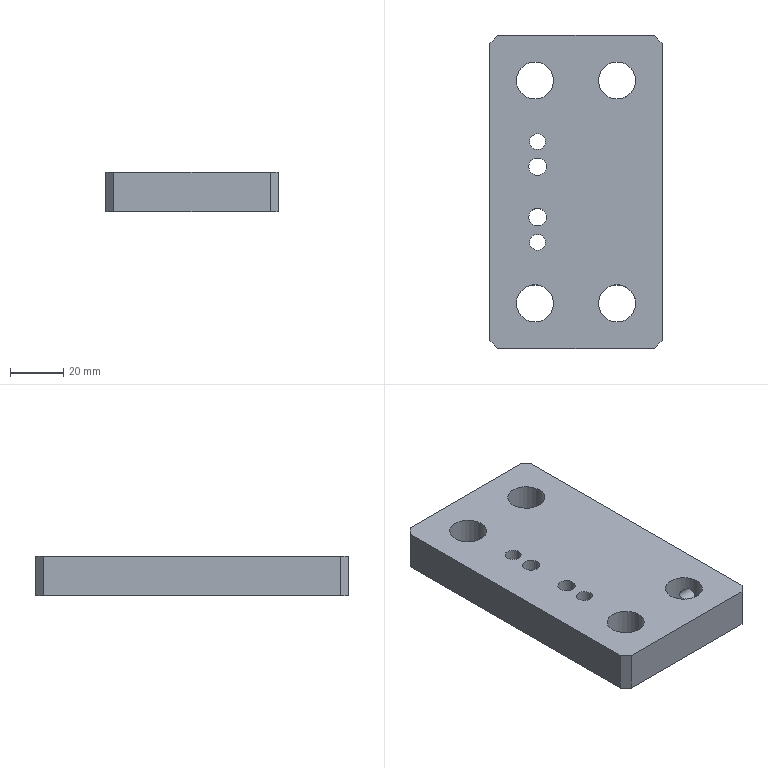Part | NX | features BREP 1 | 1 solid | 26 faces | box 65 x 118 x 15 mm | volume 102149 mm3 | cylinder 13 | plane 12 | cone 1 | commonest cylinder face diameters 14 x4 5 x3 6 x2 6.6 x2 11 x2
STEP:
#1=CARTESIAN_POINT('',(32.5,-38.5,5.));
#2=VERTEX_POINT('',#1);
#3=CARTESIAN_POINT('',(32.5,-38.5,7.5));
#4=DIRECTION('',(1.,0.,0.));
#5=DIRECTION('',(0.,0.,-1.));
#6=AXIS2_PLACEMENT_3D('',#3,#4,#5);
#7=CIRCLE('',#6,2.5);
#8=EDGE_CURVE('',#2,#2,#7,.T.);
#9=ORIENTED_EDGE('',*,*,#8,.F.);
#10=EDGE_LOOP('',(#9));
#11=FACE_BOUND('',#10,.T.);
#12=CARTESIAN_POINT('',(32.5,38.5,5.));
#13=VERTEX_POINT('',#12);
#14=CARTESIAN_POINT('',(32.5,38.5,7.5));
#15=DIRECTION('',(1.,0.,0.));
#16=DIRECTION('',(0.,0.,-1.));
#17=AXIS2_PLACEMENT_3D('',#14,#15,#16);
#18=CIRCLE('',#17,2.5);
#19=EDGE_CURVE('',#13,#13,#18,.T.);
#20=ORIENTED_EDGE('',*,*,#19,.F.);
#21=EDGE_LOOP('',(#20));
#22=FACE_BOUND('',#21,.T.);
#23=CARTESIAN_POINT('',(32.5,-56.,15.));
#24=VERTEX_POINT('',#23);
#25=CARTESIAN_POINT('',(32.5,56.,15.));
#26=VERTEX_POINT('',#25);
#27=CARTESIAN_POINT('',(32.5,59.,15.));
#28=DIRECTION('',(0.,1.,0.));
#29=VECTOR('',#28,1000.);
#30=LINE('',#27,#29);
#31=EDGE_CURVE('',#24,#26,#30,.T.);
#32=ORIENTED_EDGE('',*,*,#31,.F.);
#33=CARTESIAN_POINT('',(32.5,-56.,0.));
#34=VERTEX_POINT('',#33);
#35=CARTESIAN_POINT('',(32.5,-56.,15.));
#36=DIRECTION('',(0.,0.,-1.));
#37=VECTOR('',#36,1000.);
#38=LINE('',#35,#37);
#39=EDGE_CURVE('',#24,#34,#38,.T.);
#40=ORIENTED_EDGE('',*,*,#39,.T.);
#41=CARTESIAN_POINT('',(32.5,56.,0.));
#42=VERTEX_POINT('',#41);
#43=CARTESIAN_POINT('',(32.5,59.,0.));
#44=DIRECTION('',(0.,1.,0.));
#45=VECTOR('',#44,1000.);
#46=LINE('',#43,#45);
#47=EDGE_CURVE('',#34,#42,#46,.T.);
#48=ORIENTED_EDGE('',*,*,#47,.T.);
#49=CARTESIAN_POINT('',(32.5,56.,15.));
#50=DIRECTION('',(0.,0.,1.));
#51=VECTOR('',#50,1000.);
#52=LINE('',#49,#51);
#53=EDGE_CURVE('',#42,#26,#52,.T.);
#54=ORIENTED_EDGE('',*,*,#53,.T.);
#55=EDGE_LOOP('',(#32,#40,#48,#54));
#56=FACE_BOUND('',#55,.T.);
#57=CARTESIAN_POINT('',(32.5,59.,15.));
#58=DIRECTION('',(-1.,0.,0.));
#59=DIRECTION('',(0.,1.,0.));
#60=AXIS2_PLACEMENT_3D('',#57,#58,#59);
#61=PLANE('',#60);
#62=ADVANCED_FACE('',(#11,#22,#56),#61,.F.);
#63=CARTESIAN_POINT('',(0.,59.,10.));
#64=VERTEX_POINT('',#63);
#65=CARTESIAN_POINT('',(0.,59.,7.5));
#66=DIRECTION('',(0.,1.,0.));
#67=DIRECTION('',(0.,0.,1.));
#68=AXIS2_PLACEMENT_3D('',#65,#66,#67);
#69=CIRCLE('',#68,2.5);
#70=EDGE_CURVE('',#64,#64,#69,.T.);
#71=ORIENTED_EDGE('',*,*,#70,.F.);
#72=EDGE_LOOP('',(#71));
#73=FACE_BOUND('',#72,.T.);
#74=CARTESIAN_POINT('',(29.5,59.,0.));
#75=VERTEX_POINT('',#74);
#76=CARTESIAN_POINT('',(-29.5,59.,0.));
#77=VERTEX_POINT('',#76);
#78=CARTESIAN_POINT('',(-32.5,59.,0.));
#79=DIRECTION('',(-1.,0.,0.));
#80=VECTOR('',#79,1000.);
#81=LINE('',#78,#80);
#82=EDGE_CURVE('',#75,#77,#81,.T.);
#83=ORIENTED_EDGE('',*,*,#82,.T.);
#84=CARTESIAN_POINT('',(-29.5,59.,15.));
#85=VERTEX_POINT('',#84);
#86=CARTESIAN_POINT('',(-29.5,59.,15.));
#87=DIRECTION('',(0.,0.,1.));
#88=VECTOR('',#87,1000.);
#89=LINE('',#86,#88);
#90=EDGE_CURVE('',#77,#85,#89,.T.);
#91=ORIENTED_EDGE('',*,*,#90,.T.);
#92=CARTESIAN_POINT('',(29.5,59.,15.));
#93=VERTEX_POINT('',#92);
#94=CARTESIAN_POINT('',(-32.5,59.,15.));
#95=DIRECTION('',(-1.,0.,0.));
#96=VECTOR('',#95,1000.);
#97=LINE('',#94,#96);
#98=EDGE_CURVE('',#93,#85,#97,.T.);
#99=ORIENTED_EDGE('',*,*,#98,.F.);
#100=CARTESIAN_POINT('',(29.5,59.,15.));
#101=DIRECTION('',(0.,0.,-1.));
#102=VECTOR('',#101,1000.);
#103=LINE('',#100,#102);
#104=EDGE_CURVE('',#93,#75,#103,.T.);
#105=ORIENTED_EDGE('',*,*,#104,.T.);
#106=EDGE_LOOP('',(#83,#91,#99,#105));
#107=FACE_BOUND('',#106,.T.);
#108=CARTESIAN_POINT('',(-32.5,59.,15.));
#109=DIRECTION('',(0.,-1.,0.));
#110=DIRECTION('',(0.,0.,1.));
#111=AXIS2_PLACEMENT_3D('',#108,#109,#110);
#112=PLANE('',#111);
#113=ADVANCED_FACE('',(#73,#107),#112,.F.);
#114=CARTESIAN_POINT('',(-32.5,56.,0.));
#115=VERTEX_POINT('',#114);
#116=CARTESIAN_POINT('',(-32.5,-56.,0.));
#117=VERTEX_POINT('',#116);
#118=CARTESIAN_POINT('',(-32.5,59.,0.));
#119=DIRECTION('',(0.,-1.,0.));
#120=VECTOR('',#119,1000.);
#121=LINE('',#118,#120);
#122=EDGE_CURVE('',#115,#117,#121,.T.);
#123=ORIENTED_EDGE('',*,*,#122,.T.);
#124=CARTESIAN_POINT('',(-32.5,-56.,15.));
#125=VERTEX_POINT('',#124);
#126=CARTESIAN_POINT('',(-32.5,-56.,15.));
#127=DIRECTION('',(0.,0.,1.));
#128=VECTOR('',#127,1000.);
#129=LINE('',#126,#128);
#130=EDGE_CURVE('',#117,#125,#129,.T.);
#131=ORIENTED_EDGE('',*,*,#130,.T.);
#132=CARTESIAN_POINT('',(-32.5,56.,15.));
#133=VERTEX_POINT('',#132);
#134=CARTESIAN_POINT('',(-32.5,59.,15.));
#135=DIRECTION('',(0.,-1.,0.));
#136=VECTOR('',#135,1000.);
#137=LINE('',#134,#136);
#138=EDGE_CURVE('',#133,#125,#137,.T.);
#139=ORIENTED_EDGE('',*,*,#138,.F.);
#140=CARTESIAN_POINT('',(-32.5,56.,15.));
#141=DIRECTION('',(0.,0.,-1.));
#142=VECTOR('',#141,1000.);
#143=LINE('',#140,#142);
#144=EDGE_CURVE('',#133,#115,#143,.T.);
#145=ORIENTED_EDGE('',*,*,#144,.T.);
#146=EDGE_LOOP('',(#123,#131,#139,#145));
#147=FACE_BOUND('',#146,.T.);
#148=CARTESIAN_POINT('',(-32.5,59.,15.));
#149=DIRECTION('',(1.,0.,0.));
#150=DIRECTION('',(0.,-1.,0.));
#151=AXIS2_PLACEMENT_3D('',#148,#149,#150);
#152=PLANE('',#151);
#153=ADVANCED_FACE('',(#147),#152,.F.);
#154=CARTESIAN_POINT('',(-29.5,-59.,15.));
#155=VERTEX_POINT('',#154);
#156=CARTESIAN_POINT('',(29.5,-59.,15.));
#157=VERTEX_POINT('',#156);
#158=CARTESIAN_POINT('',(-32.5,-59.,15.));
#159=DIRECTION('',(1.,0.,0.));
#160=VECTOR('',#159,1000.);
#161=LINE('',#158,#160);
#162=EDGE_CURVE('',#155,#157,#161,.T.);
#163=ORIENTED_EDGE('',*,*,#162,.F.);
#164=CARTESIAN_POINT('',(-29.5,-59.,0.));
#165=VERTEX_POINT('',#164);
#166=CARTESIAN_POINT('',(-29.5,-59.,15.));
#167=DIRECTION('',(0.,0.,-1.));
#168=VECTOR('',#167,1000.);
#169=LINE('',#166,#168);
#170=EDGE_CURVE('',#155,#165,#169,.T.);
#171=ORIENTED_EDGE('',*,*,#170,.T.);
#172=CARTESIAN_POINT('',(29.5,-59.,0.));
#173=VERTEX_POINT('',#172);
#174=CARTESIAN_POINT('',(-32.5,-59.,0.));
#175=DIRECTION('',(1.,0.,0.));
#176=VECTOR('',#175,1000.);
#177=LINE('',#174,#176);
#178=EDGE_CURVE('',#165,#173,#177,.T.);
#179=ORIENTED_EDGE('',*,*,#178,.T.);
#180=CARTESIAN_POINT('',(29.5,-59.,15.));
#181=DIRECTION('',(0.,0.,1.));
#182=VECTOR('',#181,1000.);
#183=LINE('',#180,#182);
#184=EDGE_CURVE('',#173,#157,#183,.T.);
#185=ORIENTED_EDGE('',*,*,#184,.T.);
#186=EDGE_LOOP('',(#163,#171,#179,#185));
#187=FACE_BOUND('',#186,.T.);
#188=CARTESIAN_POINT('',(-32.5,-59.,15.));
#189=DIRECTION('',(0.,1.,0.));
#190=DIRECTION('',(0.,0.,-1.));
#191=AXIS2_PLACEMENT_3D('',#188,#189,#190);
#192=PLANE('',#191);
#193=ADVANCED_FACE('',(#187),#192,.F.);
#194=CARTESIAN_POINT('',(-17.8,9.5,15.));
#195=VERTEX_POINT('',#194);
#196=CARTESIAN_POINT('',(-14.5,9.5,15.));
#197=DIRECTION('',(0.,0.,-1.));
#198=DIRECTION('',(-1.,0.,0.));
#199=AXIS2_PLACEMENT_3D('',#196,#197,#198);
#200=CIRCLE('',#199,3.3);
#201=EDGE_CURVE('',#195,#195,#200,.T.);
#202=ORIENTED_EDGE('',*,*,#201,.T.);
#203=EDGE_LOOP('',(#202));
#204=FACE_BOUND('',#203,.T.);
#205=CARTESIAN_POINT('',(-17.8,-9.5,15.));
#206=VERTEX_POINT('',#205);
#207=CARTESIAN_POINT('',(-14.5,-9.5,15.));
#208=DIRECTION('',(0.,0.,-1.));
#209=DIRECTION('',(-1.,0.,0.));
#210=AXIS2_PLACEMENT_3D('',#207,#208,#209);
#211=CIRCLE('',#210,3.3);
#212=EDGE_CURVE('',#206,#206,#211,.T.);
#213=ORIENTED_EDGE('',*,*,#212,.T.);
#214=EDGE_LOOP('',(#213));
#215=FACE_BOUND('',#214,.T.);
#216=CARTESIAN_POINT('',(-11.5,19.,15.));
#217=VERTEX_POINT('',#216);
#218=CARTESIAN_POINT('',(-14.5,19.,15.));
#219=DIRECTION('',(0.,0.,1.));
#220=DIRECTION('',(1.,0.,0.));
#221=AXIS2_PLACEMENT_3D('',#218,#219,#220);
#222=CIRCLE('',#221,3.);
#223=EDGE_CURVE('',#217,#217,#222,.T.);
#224=ORIENTED_EDGE('',*,*,#223,.F.);
#225=EDGE_LOOP('',(#224));
#226=FACE_BOUND('',#225,.T.);
#227=CARTESIAN_POINT('',(-11.5,-19.,15.));
#228=VERTEX_POINT('',#227);
#229=CARTESIAN_POINT('',(-14.5,-19.,15.));
#230=DIRECTION('',(0.,0.,1.));
#231=DIRECTION('',(1.,0.,0.));
#232=AXIS2_PLACEMENT_3D('',#229,#230,#231);
#233=CIRCLE('',#232,3.);
#234=EDGE_CURVE('',#228,#228,#233,.T.);
#235=ORIENTED_EDGE('',*,*,#234,.F.);
#236=EDGE_LOOP('',(#235));
#237=FACE_BOUND('',#236,.T.);
#238=CARTESIAN_POINT('',(-8.5,42.,15.));
#239=VERTEX_POINT('',#238);
#240=CARTESIAN_POINT('',(-15.5,42.,15.));
#241=DIRECTION('',(0.,0.,1.));
#242=DIRECTION('',(1.,0.,0.));
#243=AXIS2_PLACEMENT_3D('',#240,#241,#242);
#244=CIRCLE('',#243,7.);
#245=EDGE_CURVE('',#239,#239,#244,.T.);
#246=ORIENTED_EDGE('',*,*,#245,.F.);
#247=EDGE_LOOP('',(#246));
#248=FACE_BOUND('',#247,.T.);
#249=CARTESIAN_POINT('',(22.5,42.,15.));
#250=VERTEX_POINT('',#249);
#251=CARTESIAN_POINT('',(15.5,42.,15.));
#252=DIRECTION('',(0.,0.,1.));
#253=DIRECTION('',(1.,0.,0.));
#254=AXIS2_PLACEMENT_3D('',#251,#252,#253);
#255=CIRCLE('',#254,7.);
#256=EDGE_CURVE('',#250,#250,#255,.T.);
#257=ORIENTED_EDGE('',*,*,#256,.F.);
#258=EDGE_LOOP('',(#257));
#259=FACE_BOUND('',#258,.T.);
#260=CARTESIAN_POINT('',(-8.5,-42.,15.));
#261=VERTEX_POINT('',#260);
#262=CARTESIAN_POINT('',(-15.5,-42.,15.));
#263=DIRECTION('',(0.,0.,1.));
#264=DIRECTION('',(1.,0.,0.));
#265=AXIS2_PLACEMENT_3D('',#262,#263,#264);
#266=CIRCLE('',#265,7.);
#267=EDGE_CURVE('',#261,#261,#266,.T.);
#268=ORIENTED_EDGE('',*,*,#267,.F.);
#269=EDGE_LOOP('',(#268));
#270=FACE_BOUND('',#269,.T.);
#271=CARTESIAN_POINT('',(22.5,-42.,15.));
#272=VERTEX_POINT('',#271);
#273=CARTESIAN_POINT('',(15.5,-42.,15.));
#274=DIRECTION('',(0.,0.,1.));
#275=DIRECTION('',(1.,0.,0.));
#276=AXIS2_PLACEMENT_3D('',#273,#274,#275);
#277=CIRCLE('',#276,7.);
#278=EDGE_CURVE('',#272,#272,#277,.T.);
#279=ORIENTED_EDGE('',*,*,#278,.F.);
#280=EDGE_LOOP('',(#279));
#281=FACE_BOUND('',#280,.T.);
#282=ORIENTED_EDGE('',*,*,#138,.T.);
#283=CARTESIAN_POINT('',(-44.25,-44.25,15.));
#284=DIRECTION('',(0.7071,-0.7071,0.));
#285=VECTOR('',#284,1000.);
#286=LINE('',#283,#285);
#287=EDGE_CURVE('',#125,#155,#286,.T.);
#288=ORIENTED_EDGE('',*,*,#287,.T.);
#289=ORIENTED_EDGE('',*,*,#162,.T.);
#290=CARTESIAN_POINT('',(44.25,-44.25,15.));
#291=DIRECTION('',(0.7071,0.7071,0.));
#292=VECTOR('',#291,1000.);
#293=LINE('',#290,#292);
#294=EDGE_CURVE('',#157,#24,#293,.T.);
#295=ORIENTED_EDGE('',*,*,#294,.T.);
#296=ORIENTED_EDGE('',*,*,#31,.T.);
#297=CARTESIAN_POINT('',(44.25,44.25,15.));
#298=DIRECTION('',(-0.7071,0.7071,0.));
#299=VECTOR('',#298,1000.);
#300=LINE('',#297,#299);
#301=EDGE_CURVE('',#26,#93,#300,.T.);
#302=ORIENTED_EDGE('',*,*,#301,.T.);
#303=ORIENTED_EDGE('',*,*,#98,.T.);
#304=CARTESIAN_POINT('',(-44.25,44.25,15.));
#305=DIRECTION('',(-0.7071,-0.7071,0.));
#306=VECTOR('',#305,1000.);
#307=LINE('',#304,#306);
#308=EDGE_CURVE('',#85,#133,#307,.T.);
#309=ORIENTED_EDGE('',*,*,#308,.T.);
#310=EDGE_LOOP('',(#282,#288,#289,#295,#296,#302,#303,#309));
#311=FACE_BOUND('',#310,.T.);
#312=CARTESIAN_POINT('',(0.,0.,15.));
#313=DIRECTION('',(0.,0.,1.));
#314=DIRECTION('',(-1.,0.,0.));
#315=AXIS2_PLACEMENT_3D('',#312,#313,#314);
#316=PLANE('',#315);
#317=ADVANCED_FACE('',(#204,#215,#226,#237,#248,#259,#270,#281,#311),#316,.T.);
#318=CARTESIAN_POINT('',(-20.,9.5,0.));
#319=VERTEX_POINT('',#318);
#320=CARTESIAN_POINT('',(-14.5,9.5,0.));
#321=DIRECTION('',(0.,0.,-1.));
#322=DIRECTION('',(-1.,0.,0.));
#323=AXIS2_PLACEMENT_3D('',#320,#321,#322);
#324=CIRCLE('',#323,5.5);
#325=EDGE_CURVE('',#319,#319,#324,.T.);
#326=ORIENTED_EDGE('',*,*,#325,.F.);
#327=EDGE_LOOP('',(#326));
#328=FACE_BOUND('',#327,.T.);
#329=CARTESIAN_POINT('',(-20.,-9.5,0.));
#330=VERTEX_POINT('',#329);
#331=CARTESIAN_POINT('',(-14.5,-9.5,0.));
#332=DIRECTION('',(0.,0.,-1.));
#333=DIRECTION('',(-1.,0.,0.));
#334=AXIS2_PLACEMENT_3D('',#331,#332,#333);
#335=CIRCLE('',#334,5.5);
#336=EDGE_CURVE('',#330,#330,#335,.T.);
#337=ORIENTED_EDGE('',*,*,#336,.F.);
#338=EDGE_LOOP('',(#337));
#339=FACE_BOUND('',#338,.T.);
#340=CARTESIAN_POINT('',(-11.5,19.,0.));
#341=VERTEX_POINT('',#340);
#342=CARTESIAN_POINT('',(-14.5,19.,0.));
#343=DIRECTION('',(0.,0.,1.));
#344=DIRECTION('',(1.,0.,0.));
#345=AXIS2_PLACEMENT_3D('',#342,#343,#344);
#346=CIRCLE('',#345,3.);
#347=EDGE_CURVE('',#341,#341,#346,.T.);
#348=ORIENTED_EDGE('',*,*,#347,.T.);
#349=EDGE_LOOP('',(#348));
#350=FACE_BOUND('',#349,.T.);
#351=CARTESIAN_POINT('',(-11.5,-19.,0.));
#352=VERTEX_POINT('',#351);
#353=CARTESIAN_POINT('',(-14.5,-19.,0.));
#354=DIRECTION('',(0.,0.,1.));
#355=DIRECTION('',(1.,0.,0.));
#356=AXIS2_PLACEMENT_3D('',#353,#354,#355);
#357=CIRCLE('',#356,3.);
#358=EDGE_CURVE('',#352,#352,#357,.T.);
#359=ORIENTED_EDGE('',*,*,#358,.T.);
#360=EDGE_LOOP('',(#359));
#361=FACE_BOUND('',#360,.T.);
#362=CARTESIAN_POINT('',(-8.5,42.,0.));
#363=VERTEX_POINT('',#362);
#364=CARTESIAN_POINT('',(-15.5,42.,0.));
#365=DIRECTION('',(0.,0.,1.));
#366=DIRECTION('',(1.,0.,0.));
#367=AXIS2_PLACEMENT_3D('',#364,#365,#366);
#368=CIRCLE('',#367,7.);
#369=EDGE_CURVE('',#363,#363,#368,.T.);
#370=ORIENTED_EDGE('',*,*,#369,.T.);
#371=EDGE_LOOP('',(#370));
#372=FACE_BOUND('',#371,.T.);
#373=CARTESIAN_POINT('',(22.5,42.,0.));
#374=VERTEX_POINT('',#373);
#375=CARTESIAN_POINT('',(15.5,42.,0.));
#376=DIRECTION('',(0.,0.,1.));
#377=DIRECTION('',(1.,0.,0.));
#378=AXIS2_PLACEMENT_3D('',#375,#376,#377);
#379=CIRCLE('',#378,7.);
#380=EDGE_CURVE('',#374,#374,#379,.T.);
#381=ORIENTED_EDGE('',*,*,#380,.T.);
#382=EDGE_LOOP('',(#381));
#383=FACE_BOUND('',#382,.T.);
#384=CARTESIAN_POINT('',(-8.5,-42.,0.));
#385=VERTEX_POINT('',#384);
#386=CARTESIAN_POINT('',(-15.5,-42.,0.));
#387=DIRECTION('',(0.,0.,1.));
#388=DIRECTION('',(1.,0.,0.));
#389=AXIS2_PLACEMENT_3D('',#386,#387,#388);
#390=CIRCLE('',#389,7.);
#391=EDGE_CURVE('',#385,#385,#390,.T.);
#392=ORIENTED_EDGE('',*,*,#391,.T.);
#393=EDGE_LOOP('',(#392));
#394=FACE_BOUND('',#393,.T.);
#395=CARTESIAN_POINT('',(22.5,-42.,0.));
#396=VERTEX_POINT('',#395);
#397=CARTESIAN_POINT('',(15.5,-42.,0.));
#398=DIRECTION('',(0.,0.,1.));
#399=DIRECTION('',(1.,0.,0.));
#400=AXIS2_PLACEMENT_3D('',#397,#398,#399);
#401=CIRCLE('',#400,7.);
#402=EDGE_CURVE('',#396,#396,#401,.T.);
#403=ORIENTED_EDGE('',*,*,#402,.T.);
#404=EDGE_LOOP('',(#403));
#405=FACE_BOUND('',#404,.T.);
#406=ORIENTED_EDGE('',*,*,#178,.F.);
#407=CARTESIAN_POINT('',(-29.5,-59.,0.));
#408=DIRECTION('',(-0.7071,0.7071,0.));
#409=VECTOR('',#408,1000.);
#410=LINE('',#407,#409);
#411=EDGE_CURVE('',#165,#117,#410,.T.);
#412=ORIENTED_EDGE('',*,*,#411,.T.);
#413=ORIENTED_EDGE('',*,*,#122,.F.);
#414=CARTESIAN_POINT('',(-32.5,56.,0.));
#415=DIRECTION('',(0.7071,0.7071,0.));
#416=VECTOR('',#415,1000.);
#417=LINE('',#414,#416);
#418=EDGE_CURVE('',#115,#77,#417,.T.);
#419=ORIENTED_EDGE('',*,*,#418,.T.);
#420=ORIENTED_EDGE('',*,*,#82,.F.);
#421=CARTESIAN_POINT('',(29.5,59.,0.));
#422=DIRECTION('',(0.7071,-0.7071,0.));
#423=VECTOR('',#422,1000.);
#424=LINE('',#421,#423);
#425=EDGE_CURVE('',#75,#42,#424,.T.);
#426=ORIENTED_EDGE('',*,*,#425,.T.);
#427=ORIENTED_EDGE('',*,*,#47,.F.);
#428=CARTESIAN_POINT('',(32.5,-56.,0.));
#429=DIRECTION('',(-0.7071,-0.7071,0.));
#430=VECTOR('',#429,1000.);
#431=LINE('',#428,#430);
#432=EDGE_CURVE('',#34,#173,#431,.T.);
#433=ORIENTED_EDGE('',*,*,#432,.T.);
#434=EDGE_LOOP('',(#406,#412,#413,#419,#420,#426,#427,#433));
#435=FACE_BOUND('',#434,.T.);
#436=CARTESIAN_POINT('',(0.,0.,0.));
#437=DIRECTION('',(0.,0.,1.));
#438=DIRECTION('',(-1.,0.,0.));
#439=AXIS2_PLACEMENT_3D('',#436,#437,#438);
#440=PLANE('',#439);
#441=ADVANCED_FACE('',(#328,#339,#350,#361,#372,#383,#394,#405,#435),#440,.F.);
#442=CARTESIAN_POINT('',(21.562,-38.5,5.));
#443=VERTEX_POINT('',#442);
#444=CARTESIAN_POINT('',(22.415,-40.562,5.55));
#445=CARTESIAN_POINT('',(21.797,-38.777,4.873));
#446=CARTESIAN_POINT('',(20.968,-37.589,5.119));
#447=CARTESIAN_POINT('',(20.271,-36.848,5.562));
#448=CARTESIAN_POINT('',(19.587,-36.297,6.21));
#449=CARTESIAN_POINT('',(19.006,-35.94,7.157));
#450=CARTESIAN_POINT('',(19.213,-36.059,8.31));
#451=CARTESIAN_POINT('',(19.88,-36.514,9.092));
#452=CARTESIAN_POINT('',(20.572,-37.144,9.655));
#453=CARTESIAN_POINT('',(21.469,-38.21,10.11));
#454=CARTESIAN_POINT('',(22.306,-39.988,9.896));
#455=CARTESIAN_POINT('',(22.458,-41.332,7.866));
#456=CARTESIAN_POINT('',(22.415,-40.562,5.55));
#457=CARTESIAN_POINT('',(21.797,-38.777,4.873));
#458=CARTESIAN_POINT('',(20.968,-37.589,5.119));
#459=B_SPLINE_CURVE_WITH_KNOTS('',3,(#444,#445,#446,#447,#448,#449,#450,#451,#452,#453,#454,#455,#456,#457,#458),.UNSPECIFIED.,.T.,.F.,(1,1,1,1,1,1,1,1,1,1,1,1,1,1,1,1,1,1,1),(-0.006513,-0.004342,-0.002171,0.,0.001085,0.002171,0.003256,0.004342,0.005427,0.006513,0.007598,0.008683,0.01085,0.01303,0.0152,0.01737,0.01845,0.01954,0.02062),.UNSPECIFIED.);
#460=EDGE_CURVE('',#443,#443,#459,.T.);
#461=ORIENTED_EDGE('',*,*,#460,.T.);
#462=EDGE_LOOP('',(#461));
#463=FACE_BOUND('',#462,.T.);
#464=ORIENTED_EDGE('',*,*,#402,.F.);
#465=EDGE_LOOP('',(#464));
#466=FACE_BOUND('',#465,.T.);
#467=ORIENTED_EDGE('',*,*,#278,.T.);
#468=EDGE_LOOP('',(#467));
#469=FACE_BOUND('',#468,.T.);
#470=CARTESIAN_POINT('',(15.5,-42.,15.));
#471=DIRECTION('',(0.,0.,1.));
#472=DIRECTION('',(-1.,0.,0.));
#473=AXIS2_PLACEMENT_3D('',#470,#471,#472);
#474=CYLINDRICAL_SURFACE('',#473,7.);
#475=ADVANCED_FACE('',(#463,#466,#469),#474,.F.);
#476=ORIENTED_EDGE('',*,*,#391,.F.);
#477=EDGE_LOOP('',(#476));
#478=FACE_BOUND('',#477,.T.);
#479=ORIENTED_EDGE('',*,*,#267,.T.);
#480=EDGE_LOOP('',(#479));
#481=FACE_BOUND('',#480,.T.);
#482=CARTESIAN_POINT('',(-15.5,-42.,15.));
#483=DIRECTION('',(0.,0.,1.));
#484=DIRECTION('',(-1.,0.,0.));
#485=AXIS2_PLACEMENT_3D('',#482,#483,#484);
#486=CYLINDRICAL_SURFACE('',#485,7.);
#487=ADVANCED_FACE('',(#478,#481),#486,.F.);
#488=CARTESIAN_POINT('',(21.562,38.5,5.));
#489=VERTEX_POINT('',#488);
#490=CARTESIAN_POINT('',(20.964,37.584,5.121));
#491=CARTESIAN_POINT('',(21.8,38.781,4.873));
#492=CARTESIAN_POINT('',(22.412,40.552,5.543));
#493=CARTESIAN_POINT('',(22.458,41.332,7.855));
#494=CARTESIAN_POINT('',(22.31,40.004,9.885));
#495=CARTESIAN_POINT('',(21.475,38.218,10.112));
#496=CARTESIAN_POINT('',(20.573,37.144,9.656));
#497=CARTESIAN_POINT('',(19.877,36.511,9.089));
#498=CARTESIAN_POINT('',(19.211,36.057,8.307));
#499=CARTESIAN_POINT('',(19.007,35.941,7.152));
#500=CARTESIAN_POINT('',(19.588,36.298,6.209));
#501=CARTESIAN_POINT('',(20.272,36.849,5.562));
#502=CARTESIAN_POINT('',(20.964,37.584,5.121));
#503=CARTESIAN_POINT('',(21.8,38.781,4.873));
#504=CARTESIAN_POINT('',(22.412,40.552,5.543));
#505=B_SPLINE_CURVE_WITH_KNOTS('',3,(#490,#491,#492,#493,#494,#495,#496,#497,#498,#499,#500,#501,#502,#503,#504),.UNSPECIFIED.,.T.,.F.,(1,1,1,1,1,1,1,1,1,1,1,1,1,1,1,1,1,1,1),(-0.003271,-0.002181,-0.00109,0.,0.002181,0.004362,0.006543,0.008723,0.009814,0.0109,0.01199,0.01309,0.01418,0.01527,0.01636,0.01745,0.01963,0.02181,0.02399),.UNSPECIFIED.);
#506=EDGE_CURVE('',#489,#489,#505,.T.);
#507=ORIENTED_EDGE('',*,*,#506,.T.);
#508=EDGE_LOOP('',(#507));
#509=FACE_BOUND('',#508,.T.);
#510=ORIENTED_EDGE('',*,*,#380,.F.);
#511=EDGE_LOOP('',(#510));
#512=FACE_BOUND('',#511,.T.);
#513=ORIENTED_EDGE('',*,*,#256,.T.);
#514=EDGE_LOOP('',(#513));
#515=FACE_BOUND('',#514,.T.);
#516=CARTESIAN_POINT('',(15.5,42.,15.));
#517=DIRECTION('',(0.,0.,1.));
#518=DIRECTION('',(-1.,0.,0.));
#519=AXIS2_PLACEMENT_3D('',#516,#517,#518);
#520=CYLINDRICAL_SURFACE('',#519,7.);
#521=ADVANCED_FACE('',(#509,#512,#515),#520,.F.);
#522=ORIENTED_EDGE('',*,*,#369,.F.);
#523=EDGE_LOOP('',(#522));
#524=FACE_BOUND('',#523,.T.);
#525=ORIENTED_EDGE('',*,*,#245,.T.);
#526=EDGE_LOOP('',(#525));
#527=FACE_BOUND('',#526,.T.);
#528=CARTESIAN_POINT('',(-15.5,42.,15.));
#529=DIRECTION('',(0.,0.,1.));
#530=DIRECTION('',(-1.,0.,0.));
#531=AXIS2_PLACEMENT_3D('',#528,#529,#530);
#532=CYLINDRICAL_SURFACE('',#531,7.);
#533=ADVANCED_FACE('',(#524,#527),#532,.F.);
#534=ORIENTED_EDGE('',*,*,#287,.F.);
#535=ORIENTED_EDGE('',*,*,#130,.F.);
#536=ORIENTED_EDGE('',*,*,#411,.F.);
#537=ORIENTED_EDGE('',*,*,#170,.F.);
#538=EDGE_LOOP('',(#534,#535,#536,#537));
#539=FACE_BOUND('',#538,.T.);
#540=CARTESIAN_POINT('',(-29.5,-59.,15.));
#541=DIRECTION('',(0.7071,0.7071,0.));
#542=DIRECTION('',(0.,0.,1.));
#543=AXIS2_PLACEMENT_3D('',#540,#541,#542);
#544=PLANE('',#543);
#545=ADVANCED_FACE('',(#539),#544,.F.);
#546=ORIENTED_EDGE('',*,*,#294,.F.);
#547=ORIENTED_EDGE('',*,*,#184,.F.);
#548=ORIENTED_EDGE('',*,*,#432,.F.);
#549=ORIENTED_EDGE('',*,*,#39,.F.);
#550=EDGE_LOOP('',(#546,#547,#548,#549));
#551=FACE_BOUND('',#550,.T.);
#552=CARTESIAN_POINT('',(32.5,-56.,15.));
#553=DIRECTION('',(-0.7071,0.7071,0.));
#554=DIRECTION('',(0.,0.,1.));
#555=AXIS2_PLACEMENT_3D('',#552,#553,#554);
#556=PLANE('',#555);
#557=ADVANCED_FACE('',(#551),#556,.F.);
#558=ORIENTED_EDGE('',*,*,#308,.F.);
#559=ORIENTED_EDGE('',*,*,#90,.F.);
#560=ORIENTED_EDGE('',*,*,#418,.F.);
#561=ORIENTED_EDGE('',*,*,#144,.F.);
#562=EDGE_LOOP('',(#558,#559,#560,#561));
#563=FACE_BOUND('',#562,.T.);
#564=CARTESIAN_POINT('',(-32.5,56.,15.));
#565=DIRECTION('',(0.7071,-0.7071,0.));
#566=DIRECTION('',(0.,0.,1.));
#567=AXIS2_PLACEMENT_3D('',#564,#565,#566);
#568=PLANE('',#567);
#569=ADVANCED_FACE('',(#563),#568,.F.);
#570=ORIENTED_EDGE('',*,*,#301,.F.);
#571=ORIENTED_EDGE('',*,*,#53,.F.);
#572=ORIENTED_EDGE('',*,*,#425,.F.);
#573=ORIENTED_EDGE('',*,*,#104,.F.);
#574=EDGE_LOOP('',(#570,#571,#572,#573));
#575=FACE_BOUND('',#574,.T.);
#576=CARTESIAN_POINT('',(29.5,59.,15.));
#577=DIRECTION('',(-0.7071,-0.7071,0.));
#578=DIRECTION('',(0.,0.,1.));
#579=AXIS2_PLACEMENT_3D('',#576,#577,#578);
#580=PLANE('',#579);
#581=ADVANCED_FACE('',(#575),#580,.F.);
#582=ORIENTED_EDGE('',*,*,#358,.F.);
#583=EDGE_LOOP('',(#582));
#584=FACE_BOUND('',#583,.T.);
#585=ORIENTED_EDGE('',*,*,#234,.T.);
#586=EDGE_LOOP('',(#585));
#587=FACE_BOUND('',#586,.T.);
#588=CARTESIAN_POINT('',(-14.5,-19.,15.));
#589=DIRECTION('',(0.,0.,1.));
#590=DIRECTION('',(-1.,0.,0.));
#591=AXIS2_PLACEMENT_3D('',#588,#589,#590);
#592=CYLINDRICAL_SURFACE('',#591,3.);
#593=ADVANCED_FACE('',(#584,#587),#592,.F.);
#594=ORIENTED_EDGE('',*,*,#347,.F.);
#595=EDGE_LOOP('',(#594));
#596=FACE_BOUND('',#595,.T.);
#597=ORIENTED_EDGE('',*,*,#223,.T.);
#598=EDGE_LOOP('',(#597));
#599=FACE_BOUND('',#598,.T.);
#600=CARTESIAN_POINT('',(-14.5,19.,15.));
#601=DIRECTION('',(0.,0.,1.));
#602=DIRECTION('',(-1.,0.,0.));
#603=AXIS2_PLACEMENT_3D('',#600,#601,#602);
#604=CYLINDRICAL_SURFACE('',#603,3.);
#605=ADVANCED_FACE('',(#596,#599),#604,.F.);
#606=ORIENTED_EDGE('',*,*,#212,.F.);
#607=EDGE_LOOP('',(#606));
#608=FACE_BOUND('',#607,.T.);
#609=CARTESIAN_POINT('',(-17.8,-9.5,6.4));
#610=VERTEX_POINT('',#609);
#611=CARTESIAN_POINT('',(-14.5,-9.5,6.4));
#612=DIRECTION('',(0.,0.,-1.));
#613=DIRECTION('',(-1.,0.,0.));
#614=AXIS2_PLACEMENT_3D('',#611,#612,#613);
#615=CIRCLE('',#614,3.3);
#616=EDGE_CURVE('',#610,#610,#615,.T.);
#617=ORIENTED_EDGE('',*,*,#616,.T.);
#618=EDGE_LOOP('',(#617));
#619=FACE_BOUND('',#618,.T.);
#620=CARTESIAN_POINT('',(-14.5,-9.5,0.));
#621=DIRECTION('',(0.,0.,-1.));
#622=DIRECTION('',(1.,0.,0.));
#623=AXIS2_PLACEMENT_3D('',#620,#621,#622);
#624=CYLINDRICAL_SURFACE('',#623,3.3);
#625=ADVANCED_FACE('',(#608,#619),#624,.F.);
#626=ORIENTED_EDGE('',*,*,#616,.F.);
#627=EDGE_LOOP('',(#626));
#628=FACE_BOUND('',#627,.T.);
#629=CARTESIAN_POINT('',(-20.,-9.5,6.4));
#630=VERTEX_POINT('',#629);
#631=CARTESIAN_POINT('',(-14.5,-9.5,6.4));
#632=DIRECTION('',(0.,0.,-1.));
#633=DIRECTION('',(-1.,0.,0.));
#634=AXIS2_PLACEMENT_3D('',#631,#632,#633);
#635=CIRCLE('',#634,5.5);
#636=EDGE_CURVE('',#630,#630,#635,.T.);
#637=ORIENTED_EDGE('',*,*,#636,.T.);
#638=EDGE_LOOP('',(#637));
#639=FACE_BOUND('',#638,.T.);
#640=CARTESIAN_POINT('',(-11.2,-9.5,6.4));
#641=DIRECTION('',(0.,0.,1.));
#642=DIRECTION('',(-1.,0.,0.));
#643=AXIS2_PLACEMENT_3D('',#640,#641,#642);
#644=PLANE('',#643);
#645=ADVANCED_FACE('',(#628,#639),#644,.F.);
#646=ORIENTED_EDGE('',*,*,#636,.F.);
#647=EDGE_LOOP('',(#646));
#648=FACE_BOUND('',#647,.T.);
#649=ORIENTED_EDGE('',*,*,#336,.T.);
#650=EDGE_LOOP('',(#649));
#651=FACE_BOUND('',#650,.T.);
#652=CARTESIAN_POINT('',(-14.5,-9.5,0.));
#653=DIRECTION('',(0.,0.,-1.));
#654=DIRECTION('',(1.,0.,0.));
#655=AXIS2_PLACEMENT_3D('',#652,#653,#654);
#656=CYLINDRICAL_SURFACE('',#655,5.5);
#657=ADVANCED_FACE('',(#648,#651),#656,.F.);
#658=ORIENTED_EDGE('',*,*,#201,.F.);
#659=EDGE_LOOP('',(#658));
#660=FACE_BOUND('',#659,.T.);
#661=CARTESIAN_POINT('',(-17.8,9.5,6.4));
#662=VERTEX_POINT('',#661);
#663=CARTESIAN_POINT('',(-14.5,9.5,6.4));
#664=DIRECTION('',(0.,0.,-1.));
#665=DIRECTION('',(-1.,0.,0.));
#666=AXIS2_PLACEMENT_3D('',#663,#664,#665);
#667=CIRCLE('',#666,3.3);
#668=EDGE_CURVE('',#662,#662,#667,.T.);
#669=ORIENTED_EDGE('',*,*,#668,.T.);
#670=EDGE_LOOP('',(#669));
#671=FACE_BOUND('',#670,.T.);
#672=CARTESIAN_POINT('',(-14.5,9.5,0.));
#673=DIRECTION('',(0.,0.,-1.));
#674=DIRECTION('',(1.,0.,0.));
#675=AXIS2_PLACEMENT_3D('',#672,#673,#674);
#676=CYLINDRICAL_SURFACE('',#675,3.3);
#677=ADVANCED_FACE('',(#660,#671),#676,.F.);
#678=ORIENTED_EDGE('',*,*,#668,.F.);
#679=EDGE_LOOP('',(#678));
#680=FACE_BOUND('',#679,.T.);
#681=CARTESIAN_POINT('',(-20.,9.5,6.4));
#682=VERTEX_POINT('',#681);
#683=CARTESIAN_POINT('',(-14.5,9.5,6.4));
#684=DIRECTION('',(0.,0.,-1.));
#685=DIRECTION('',(-1.,0.,0.));
#686=AXIS2_PLACEMENT_3D('',#683,#684,#685);
#687=CIRCLE('',#686,5.5);
#688=EDGE_CURVE('',#682,#682,#687,.T.);
#689=ORIENTED_EDGE('',*,*,#688,.T.);
#690=EDGE_LOOP('',(#689));
#691=FACE_BOUND('',#690,.T.);
#692=CARTESIAN_POINT('',(-11.2,9.5,6.4));
#693=DIRECTION('',(0.,0.,1.));
#694=DIRECTION('',(-1.,0.,0.));
#695=AXIS2_PLACEMENT_3D('',#692,#693,#694);
#696=PLANE('',#695);
#697=ADVANCED_FACE('',(#680,#691),#696,.F.);
#698=ORIENTED_EDGE('',*,*,#688,.F.);
#699=EDGE_LOOP('',(#698));
#700=FACE_BOUND('',#699,.T.);
#701=ORIENTED_EDGE('',*,*,#325,.T.);
#702=EDGE_LOOP('',(#701));
#703=FACE_BOUND('',#702,.T.);
#704=CARTESIAN_POINT('',(-14.5,9.5,0.));
#705=DIRECTION('',(0.,0.,-1.));
#706=DIRECTION('',(1.,0.,0.));
#707=AXIS2_PLACEMENT_3D('',#704,#705,#706);
#708=CYLINDRICAL_SURFACE('',#707,5.5);
#709=ADVANCED_FACE('',(#700,#703),#708,.F.);
#710=CARTESIAN_POINT('',(0.,42.498,7.5));
#711=VERTEX_POINT('',#710);
#712=VERTEX_LOOP('',#711);
#713=FACE_BOUND('',#712,.T.);
#714=CARTESIAN_POINT('',(0.,44.,10.));
#715=VERTEX_POINT('',#714);
#716=CARTESIAN_POINT('',(0.,44.,7.5));
#717=DIRECTION('',(0.,1.,0.));
#718=DIRECTION('',(0.,0.,1.));
#719=AXIS2_PLACEMENT_3D('',#716,#717,#718);
#720=CIRCLE('',#719,2.5);
#721=EDGE_CURVE('',#715,#715,#720,.T.);
#722=ORIENTED_EDGE('',*,*,#721,.T.);
#723=EDGE_LOOP('',(#722));
#724=FACE_BOUND('',#723,.T.);
#725=CARTESIAN_POINT('',(0.,44.,7.5));
#726=DIRECTION('',(0.,1.,0.));
#727=DIRECTION('',(0.,0.,-1.));
#728=AXIS2_PLACEMENT_3D('',#725,#726,#727);
#729=CONICAL_SURFACE('',#728,2.5,1.03);
#730=ADVANCED_FACE('',(#713,#724),#729,.F.);
#731=ORIENTED_EDGE('',*,*,#721,.F.);
#732=EDGE_LOOP('',(#731));
#733=FACE_BOUND('',#732,.T.);
#734=ORIENTED_EDGE('',*,*,#70,.T.);
#735=EDGE_LOOP('',(#734));
#736=FACE_BOUND('',#735,.T.);
#737=CARTESIAN_POINT('',(0.,59.,7.5));
#738=DIRECTION('',(0.,1.,0.));
#739=DIRECTION('',(0.,0.,-1.));
#740=AXIS2_PLACEMENT_3D('',#737,#738,#739);
#741=CYLINDRICAL_SURFACE('',#740,2.5);
#742=ADVANCED_FACE('',(#733,#736),#741,.F.);
#743=ORIENTED_EDGE('',*,*,#19,.T.);
#744=EDGE_LOOP('',(#743));
#745=FACE_BOUND('',#744,.T.);
#746=ORIENTED_EDGE('',*,*,#506,.F.);
#747=EDGE_LOOP('',(#746));
#748=FACE_BOUND('',#747,.T.);
#749=CARTESIAN_POINT('',(32.5,38.5,7.5));
#750=DIRECTION('',(1.,0.,0.));
#751=DIRECTION('',(0.,0.,1.));
#752=AXIS2_PLACEMENT_3D('',#749,#750,#751);
#753=CYLINDRICAL_SURFACE('',#752,2.5);
#754=ADVANCED_FACE('',(#745,#748),#753,.F.);
#755=ORIENTED_EDGE('',*,*,#8,.T.);
#756=EDGE_LOOP('',(#755));
#757=FACE_BOUND('',#756,.T.);
#758=ORIENTED_EDGE('',*,*,#460,.F.);
#759=EDGE_LOOP('',(#758));
#760=FACE_BOUND('',#759,.T.);
#761=CARTESIAN_POINT('',(32.5,-38.5,7.5));
#762=DIRECTION('',(1.,0.,0.));
#763=DIRECTION('',(0.,0.,1.));
#764=AXIS2_PLACEMENT_3D('',#761,#762,#763);
#765=CYLINDRICAL_SURFACE('',#764,2.5);
#766=ADVANCED_FACE('',(#757,#760),#765,.F.);
#767=CLOSED_SHELL('',(#62,#113,#153,#193,#317,#441,#475,#487,#521,#533,#545,#557,#569,#581,#593,#605,#625,#645,#657,#677,#697,#709,#730,#742,#754,#766));
#768=MANIFOLD_SOLID_BREP('',#767);
#769=(LENGTH_UNIT()NAMED_UNIT(*)SI_UNIT(.MILLI.,.METRE.));
#770=UNCERTAINTY_MEASURE_WITH_UNIT(LENGTH_MEASURE(0.0508),#769,'','');
#771=(NAMED_UNIT(*)PLANE_ANGLE_UNIT()SI_UNIT($,.RADIAN.));
#772=(NAMED_UNIT(*)SI_UNIT($,.STERADIAN.)SOLID_ANGLE_UNIT());
#773=(GEOMETRIC_REPRESENTATION_CONTEXT(3)GLOBAL_UNCERTAINTY_ASSIGNED_CONTEXT((#770))GLOBAL_UNIT_ASSIGNED_CONTEXT((#769,#771,#772))REPRESENTATION_CONTEXT('',''));
#774=ADVANCED_BREP_SHAPE_REPRESENTATION('',(#768),#773);